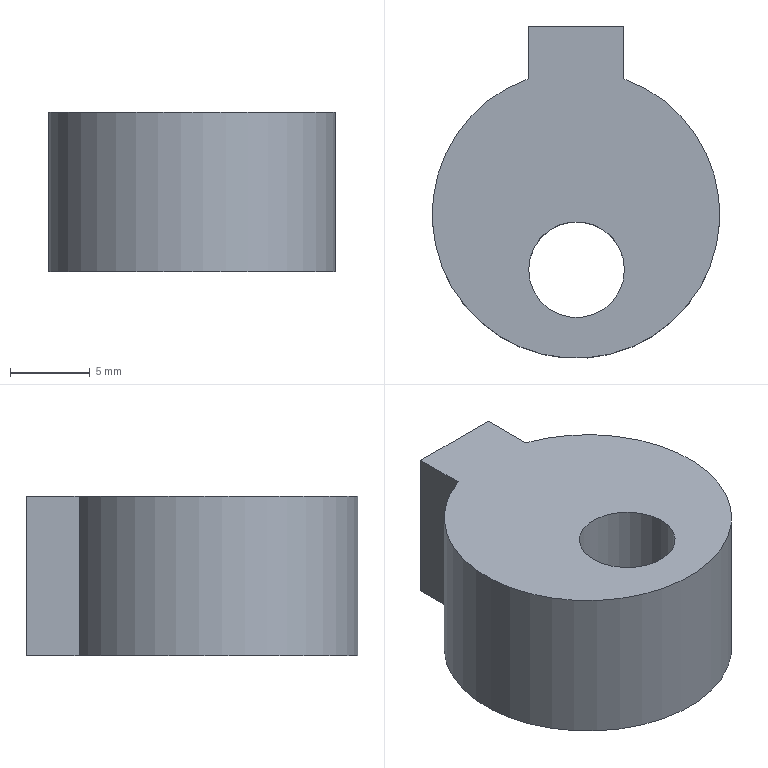NC program | NX | posted with a generic post | part box 18 x 20.8 x 10 mm
Lines 1868 to 1937 of 1937:
(PLANAR_MILL_COPY , TOOL : 倒角D8-90度)
N3710 M6
N3712 G53
N3714 G17 G0 G90 X6.892 Y9.937 S3000 M3
N3716 G43 Z20. H5
N3718 Z0.5
N3720 G94 G1 Z-1.5 F600.
N3722 G41 X6.4 Y10.023 D5
N3724 G3 X4.4 Y8.023 R2.
N3726 G2 X-4.4 Y8.023 R-10.4
N3728 G1 Y10.3
N3730 G2 X-2.9 Y11.8 R1.5
N3732 G1 X2.9
N3734 G2 X4.4 Y10.3 R1.5
N3736 G1 Y8.023
N3738 G3 X7.058 Y8.989 R2.
N3740 G40
N3742 G1 X7.188 Y9.472
N3744 Z0.5
N3746 G0 Z20.
N3748 M5
(DRILLING_COPY_2 , TOOL : 倒角D8-90度)
N3750 T01 M6
N3752 G53
N3754 G17 G0 G90 X0.035 Y-4.853 S2000 M3
N3756 G43 Z20. H1
N3758 G94 G81 G99 Z-3.2 F200. R3.
N3760 G80
N3762 G0 X0.035 Y-4.853 Z20.
N3764 M5
(PLANAR_MILL , TOOL : D6-18-D6-50-3T-FINISH)
N3766 T05 M6
N3768 G53
N3770 G17 G0 G90 X8.492 Y10.905 S3000 M3
N3772 G43 Z20. H5
N3774 Z-10.
N3776 G94 G1 Z-12. F600.
N3778 G41 X8. Y10.992 D5
N3780 G3 X6. Y8.992 R2.
N3782 G2 X-6. Y8.992 R-12.
N3784 G1 Y10.4
N3786 G2 X-3. Y13.4 R3.
N3788 G1 X3.
N3790 G2 X6. Y10.4 R3.
N3792 G1 Y8.992
N3794 G3 X8.732 Y9.724 R2.
N3796 G40
N3798 G1 X8.903 Y10.194
N3800 X8.492 Y10.905
N3802 G41 X8. Y10.992
N3804 G3 X6. Y8.992 R2.
N3806 G2 X-6. Y8.992 R-12.
N3808 G1 Y10.4
N3810 G2 X-3. Y13.4 R3.
N3812 G1 X3.
N3814 G2 X6. Y10.4 R3.
N3816 G1 Y8.992
N3818 G3 X8.732 Y9.724 R2.
N3820 G40
N3822 G1 X8.903 Y10.194
N3824 Z-10.
N3826 G0 Z20.
N3828 M5
N3830 M2